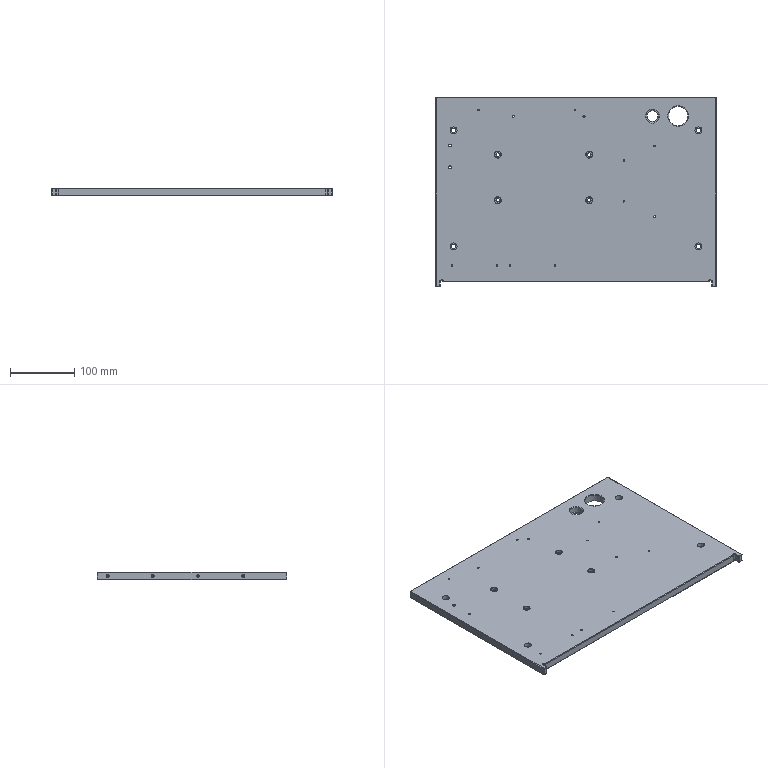CAM job | NX | 3-axis milling, drilling | part box 435 x 294.7 x 12 mm | stock box 440 x 299.7 x 12 mm
Tools:
number,name,description,diameter,corner_radius,flute_length,length,flutes
6,D6,平底铣刀-粗,6.0,0.0,25.0,75.0,2
9,D10,平底铣刀-粗,10.0,0.0,35.0,75.0,2
11,D3-J,平底铣刀-精,3.0,0.0,50.0,75.0,2
7,D6-J,平底铣刀-精,6.0,0.0,25.0,75.0,2
23,D4R0.5,圆鼻刀-粗,4.0,0.5,50.0,75.0,2
2,D6_CHAMFERMILL,倒角刀,6.0,0.0,3.0,25.0,2
20,M3X0.5,丝锥,2.5,0.0,35.0,50.0,2
21,M4X0.7,丝锥,3.3,0.0,35.0,50.0,2
22,M5X0.8,丝锥,4.2,0.0,35.0,50.0,2
12,ZT2.5,钻头,2.5,0.0,35.0,50.0,2
17,ZT5.5,钻头,5.5,0.0,35.0,50.0,2
18,ZT6.6,钻头,6.6,0.0,35.0,50.0,2
19,ZT10,钻头,10.0,0.0,35.0,50.0,2
13,DRILL3.3,Twist Drill 3.3 mm,3.3,0.0,35.0,35.008,2
14,DRILL4.2,Twist Drill 4.2 mm,4.2,0.0,41.0,41.738,2
Operations:
program,operation,operation_type,tool,method,geometry_group,spindle_rpm,surface_speed,feed_per_tooth,feed_cut,feed_plunge,cut_length_mm,path_length_mm,cut_time_min,machine_time_min
B,BOTTOMWALL_SPIRALROUGH-MID_COPY,VolumeBased25DMillingOperation,D10,LAYERROUGH-DEPTHK-STEPG,W-B,8000.0,251.327,0.125,2000.0,100.0,821.049,868.949,0.4105,0.4153
B,SPOT-DEPTH0.8,Operation,D6_CHAMFERMILL,NONE,W-B,8000.0,150.796,0.0312,500.0,90.0,41.4,1478.983,0.0828,0.2266
B,THRUHOLE-M3TAPDRILL,Operation,ZT2.5,NONE,W-B,3000.0,23.562,0.05,300.0,90.0,187.511,1205.157,0.625,0.7268
B,THRUHOLE-M4TAPDRILL,Operation,DRILL3.3,NONE,W-B,3000.0,31.102,0.05,300.0,90.0,37.983,226.97,0.1266,0.1455
B,THRUHOLE-M5TAPDRILL,Operation,DRILL4.2,NONE,W-B,3000.0,39.584,0.0583,350.0,90.0,40.524,156.062,0.1158,0.1273
B,COUNTERBORE-DRILL_SEG0,Operation,ZT5.5,NONE,W-B,1200.0,20.735,0.0625,150.0,90.0,28.0,383.018,0.1867,0.2222
B,COUNTERBORE-DRILL_SEG0_2,Operation,ZT6.6,NONE,W-B,1200.0,24.881,0.0625,150.0,90.0,32.0,847.007,0.2133,0.2948
B,MILLHOLEROUGHD6_1,CylinderMilling,D6,NONE,W-B,8000.0,150.796,0.075,1200.0,100.0,520.893,979.693,0.4341,0.48
B,MILLHOLEROUGHD6_2,CylinderMilling,D6,NONE,W-B,8000.0,150.796,0.075,1200.0,100.0,923.332,1846.932,0.7694,0.8618
B,MILLHOLEFINISHD6_1,CylinderMilling,D6-J,FINISHSTEPDEPTHOFF,W-B,8000.0,150.796,0.0312,500.0,100.0,120.611,581.411,0.2412,0.2873
B,MILLHOLEFINISHD6_2,CylinderMilling,D6-J,FINISHSTEPDEPTHOFF,W-B,8000.0,150.796,0.0312,500.0,100.0,178.461,1104.061,0.3569,0.4495
B,ZLEVELSPIRALWALL_COPY_COPY,ZLevelMilling,D4R0.5,ZLEVELWALL-DEPTHK-STEPG,W-B,7000.0,87.965,0.3571,5000.0,100.0,42334.314,42881.447,8.467,8.522
B,DRILL_CHAMFER_4,Operation,D6_CHAMFERMILL,METHOD,W-B,8000.0,150.796,0.0312,500.0,0.0,47.5,943.726,0.095,0.1846
B,DRILL_CHAMFER_5,Operation,D6_CHAMFERMILL,METHOD,W-B,8000.0,150.796,0.0312,500.0,0.0,10.4,173.841,0.0208,0.0371
B,MILL_CHAMFER_3,PlanarMilling,D6_CHAMFERMILL,METHOD,W-B,8000.0,150.796,0.0312,500.0,100.0,36.041,153.428,0.0721,0.0838
B,MILL_CHAMFER_4,PlanarMilling,D6_CHAMFERMILL,NONE,W-B,8000.0,150.796,0.05,800.0,100.0,159.312,582.492,0.1991,0.2415
B,MILL_CHAMFER_5,PlanarMilling,D6_CHAMFERMILL,NONE,W-B,8000.0,150.796,0.05,800.0,100.0,173.57,1064.64,0.217,0.3061
B,THRUHOLE-TAPM3,Operation,M3X0.5,METHOD,W-B,800.0,6.283,0.0003,0.5,90.0,160.0,1150.135,320.0,320.099
B,THRUHOLE-TAPM4,Operation,M4X0.7,METHOD,W-B,600.0,6.22,0.0006,0.7,90.0,32.0,215.005,45.714,45.733
B,THRUHOLE-TAPM5,Operation,M5X0.8,METHOD,W-B,500.0,6.597,0.0008,0.8,90.0,33.0,141.015,41.25,41.261
B,BOTTOMWALL_SIDEFINISH-MID_COPY,VolumeBased25DMillingOperation,D6-J,SIDEFINISH-DEPTHK-STEPG,W-B,8000.0,150.792,0.0625,1000.0,100.0,50.743,87.743,0.0507,0.0544
A,SPOT,Operation,D6_CHAMFERMILL,METHOD,W-A,3000.0,56.549,0.0333,200.0,0.0,37.5,1203.299,0.1875,0.3041
A,SPOT_2,Operation,D6_CHAMFERMILL,METHOD,W-A,3000.0,56.549,0.0333,200.0,0.0,20.0,870.135,0.1,0.185
A,DRILL_5,Operation,ZT5.5,METHOD,W-A,2600.0,44.925,0.0231,120.0,0.0,50.8,428.618,0.4233,0.4611
A,DRILL_6,Operation,ZT6.6,METHOD,W-A,2600.0,53.91,0.0231,120.0,0.0,50.8,884.607,0.4233,0.5067
A,DRILL_7,Operation,ZT10,METHOD,W-A,2000.0,62.832,0.03,120.0,0.0,12.5,65.0,0.1042,0.1094
A,DRILL_8,Operation,ZT10,METHOD,W-A,1500.0,47.124,0.04,120.0,0.0,12.5,65.0,0.1042,0.1094
A,ROUGHHOLED6_3,CylinderMilling,D6,METHOD,W-A,6000.0,157.0,0.25,2500.0,90.0,1305.732,1356.932,0.5226,0.5278
A,ROUGHHOLE_3,CylinderMilling,D10,METHOD,W-A,6000.0,157.0,0.25,3000.0,90.0,2133.004,2184.204,0.7112,0.7164
A,PROFILE_ROUGH_2,VolumeBased25DMillingOperation,D10,METHOD,W-A,6000.0,188.0,0.25,4000.0,80.0,39014.272,39064.272,9.754,9.759
A,BOTTOMWALL_SIDEFINISH-MID_COPY_1,VolumeBased25DMillingOperation,D6-J,SIDEFINISH-DEPTHK-STEPG,W-A,8000.0,251.32,0.0625,1000.0,100.0,82.099,122.699,0.0821,0.0862
A,HOLESIDEE6_3,CylinderMilling,D6-J,METHOD,W-A,6000.0,157.0,0.2,800.0,90.0,76.472,138.523,0.0962,0.1025
A,PROFILE_D4_CORNERCLEAN,ZLevelMilling,D3-J,METHOD,W-A,6000.0,75.0,0.25,2500.0,80.0,1167.992,1727.863,0.4675,0.5235
A,ZLEVELSPIRALWALL_COPY,ZLevelMilling,D4R0.5,ZLEVELWALL-DEPTHK-STEPG,W-A,7000.0,87.965,0.3571,5000.0,100.0,38680.47,38718.97,7.736,7.74
A,CHAMFER_2,SurfaceContour,D6_CHAMFERMILL,METHOD,W-A,6000.0,113.0,0.125,1200.0,100.0,148.139,252.899,0.1234,0.1339
A,DRILL_CHAMFER_1,Operation,D6_CHAMFERMILL,METHOD,W-A,5000.0,94.248,0.015,150.0,0.0,47.5,943.726,0.3167,0.4063
A,DRILL_CHAMFER_2,Operation,D6_CHAMFERMILL,METHOD,W-A,5000.0,94.248,0.015,150.0,0.0,15.6,334.846,0.104,0.1359
A,DRILL_CHAMFER_3,Operation,D6_CHAMFERMILL,METHOD,W-A,5000.0,94.248,0.015,150.0,0.0,11.4,99.932,0.076,0.0849
A,MILL_CHAMFER_1,PlanarMilling,D6_CHAMFERMILL,METHOD,W-A,6000.0,113.097,0.05,600.0,100.0,71.178,522.384,0.1186,0.1638
A,MILL_CHAMFER_2,PlanarMilling,D6_CHAMFERMILL,METHOD,W-A,6000.0,113.097,0.05,600.0,100.0,81.784,988.99,0.1363,0.227
A,PROFILE_SEMIFINISH_2,VolumeBased25DMillingOperation,D6-J,METHOD,W-A,6000.0,113.0,0.0833,1000.0,100.0,1494.423,1556.423,1.494,1.501
A,PROFILE_FINISH_2,VolumeBased25DMillingOperation,D6-J,METHOD,W-A,6000.0,113.0,0.0833,1000.0,100.0,1494.223,1556.823,1.494,1.5